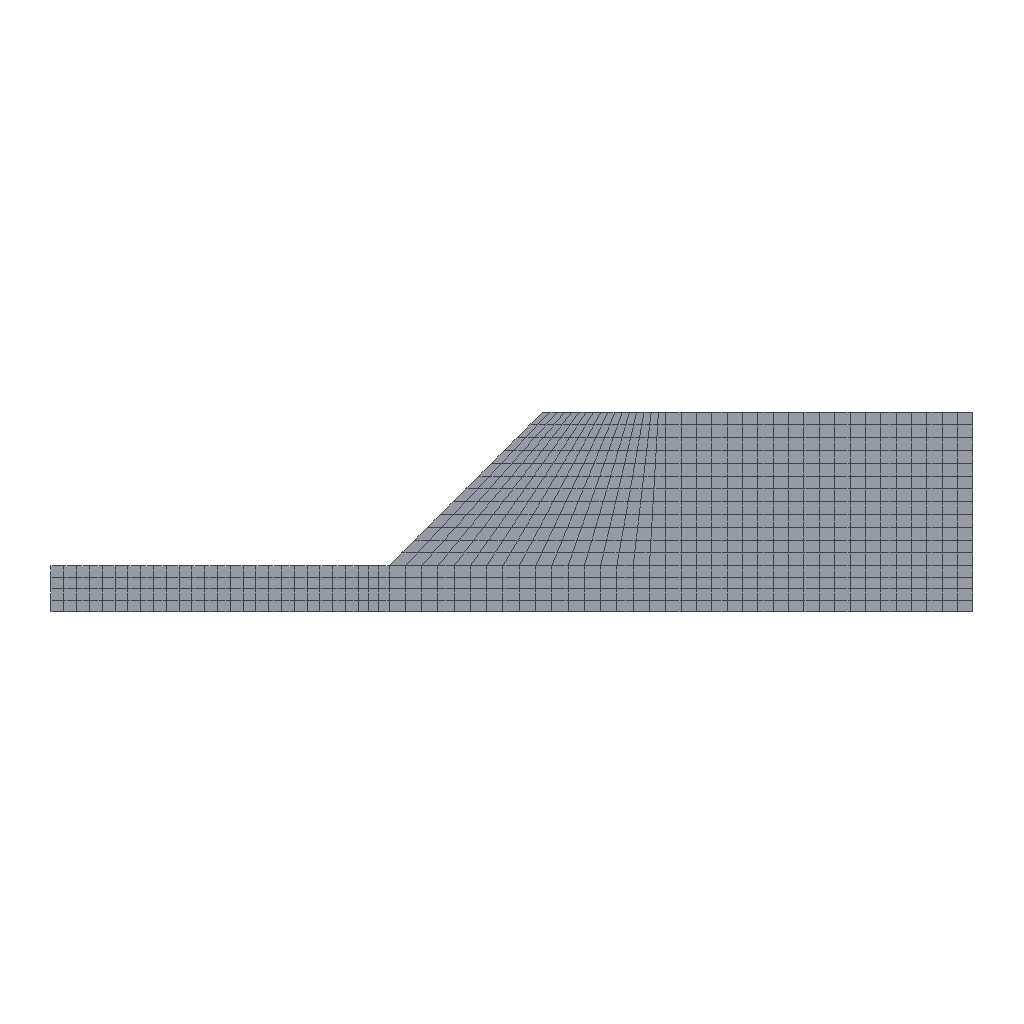Simulation study | abaqus
Set-up summary:
category,name,step,type,value,unit,region
solver,abaqus,,Abaqus/CAE 2024
units,mm-N-s-tonne (MPa),,inferred,E=10000 density=
analysis,Load,,static,time_period=1
analysis,Reduce,,static,time_period=1
mesh,nodes,,,781
mesh,elements,,,700
element_type,CPE4,,,700
material,soft,,E,10000
material,soft,,nu,0.35
material,soft,,behaviors,plastic; mohr coulomb; mohr coulomb hardening
material,soil,,E,100000
material,soil,,nu,0.35
material,soil,,behaviors,plastic; mohr coulomb; mohr coulomb hardening
section,soil,,solid section,,,_PickedSet17
section,soft,,solid section,,,_PickedSet18
load,,initial,initial condition field
load,Load-1,Load,by,-20,,_PickedSet7
bc,BC-1,initial,fixed,[dofs=x],,_PickedSet8
bc,BC-2,initial,fixed,"[dofs=x,y n=2]",,_PickedSet9
Abaqus input file, long lists of numbers shortened:
*Conflicts, Generated keywords
*Heading
** Job name: deck Model name: Model-1
** Generated by: Abaqus/CAE 2024
*Preprint, echo=NO, model=NO, history=NO, contact=NO
*Conflicts, User edited keywords
*Conflicts, End of conflict block
*Part, name=slope
*Node
      1,         -10.,           0.
      2,         -10.,           3.
** (779 more lines like these left out)
*Element, type=CPE4
 1,   1,  16, 217,  43
 2,  16,  17, 218, 217
** (698 more lines like these left out)
*Nset, nset=_PickedSet17, internal
   1,   2,   3,   4,   5,   6,   7,   8,   9,  11,  12,  15,  16,  17,  18,  19
  20,  21,  22,  23,  24,  25,  26,  27,  28,  29,  30,  31,  32,  33,  34,  35
** (39 more lines like these left out)
*Elset, elset=_PickedSet17, internal
   1,   2,   3,   4,   5,   6,   7,   8,   9,  10,  11,  12,  13,  14,  15,  16
  17,  18,  19,  20,  21,  22,  23,  24,  25,  26,  27,  28,  29,  30,  31,  32
** (34 more lines like these left out)
*Nset, nset=_PickedSet18, internal
   1,   2,   5,   6,   9,  10,  13,  14,  16,  17,  18,  44,  45,  46,  88,  89
  90,  91,  92,  93,  94,  95,  96,  97,  98,  99, 100, 101, 102, 103, 104, 105
** (9 more lines like these left out)
*Elset, elset=_PickedSet18, internal
 129, 130, 131, 132, 133, 134, 135, 136, 137, 138, 139, 140, 141, 142, 143, 144
 145, 146, 147, 148, 149, 150, 151, 152, 153, 154, 155, 156, 157, 158, 159, 160
** (6 more lines like these left out)
*Nset, nset=slope, generate
   1,  781,    1
*Elset, elset=slope, generate
   1,  700,    1
** Section: soil
*Solid Section, elset=_PickedSet17, material=soil
1.,
** Section: soft
*Solid Section, elset=_PickedSet18, material=soft
1.,
*End Part
**
**
** ASSEMBLY
**
*Assembly, name=Assembly
**
*Instance, name=slope-1, part=slope
*End Instance
**
*Nset, nset=_PickedSet7, internal, instance=slope-1, generate
   1,  781,    1
*Elset, elset=_PickedSet7, internal, instance=slope-1, generate
   1,  700,    1
*Nset, nset=_PickedSet8, internal, instance=slope-1
   3,   4,   7,   8,  12,  30,  31,  32,  66,  67,  68, 134, 135, 136, 137, 138
 139, 140, 141, 142, 143, 144
*Elset, elset=_PickedSet8, internal, instance=slope-1
  45,  46,  47,  48, 125, 126, 127, 128, 425, 426, 427, 428, 429, 430, 431, 432
 433, 434, 435, 436
*Nset, nset=_PickedSet9, internal, instance=slope-1
   1,   4,   6,   7,  10,  13,  33,  34,  35,  36,  37,  38,  39,  40,  41,  42
  43,  47,  48,  49,  50,  51,  52,  53,  54,  55,  56,  57,  58,  59,  60,  61
** (3 more lines like these left out)
*Elset, elset=_PickedSet9, internal, instance=slope-1
   1,   5,   9,  13,  17,  21,  25,  29,  33,  37,  41,  45,  52,  56,  60,  64
  68,  72,  76,  80,  84,  88,  92,  96, 100, 104, 108, 112, 116, 120, 124, 128
** (2 more lines like these left out)
*End Assembly
**
** MATERIALS
**
*Material, name=soft
*Elastic
10000., 0.35
*Mohr Coulomb, dependencies=1
0.,  0., , 0.5
0.,  0., ,  2.
*Mohr Coulomb Hardening, dependencies=1
40.,   0., , 0.25
10.,   0., ,   1.
 5.,   0., ,   2.
*Material, name=soil
*Elastic
100000., 0.35
*Mohr Coulomb, dependencies=1
   55.51,   0., , 0.25
 36.052,   0., ,  0.5
  25.887,   0., , 0.75
     20.,   0., ,   1.
 16.234,   0., , 1.25
  13.639,   0., ,  1.5
  11.749,   0., , 1.75
 10.314,   0., ,   2.
*Mohr Coulomb Hardening, dependencies=1
   49.52,   0., , 0.25
   24.76,   0., ,  0.5
 16.507,   0., , 0.75
   12.38,   0., ,   1.
   9.904,   0., , 1.25
 8.253,   0., ,  1.5
 7.074,   0., , 1.75
    6.19,   0., ,   2.
**
** BOUNDARY CONDITIONS
**
** Name: BC-1 Type: Displacement/Rotation
*Boundary
_PickedSet8, 1, 1
** Name: BC-2 Type: Displacement/Rotation
*Boundary
_PickedSet9, 1, 1
_PickedSet9, 2, 2
** ----------------------------------------------------------------
*initial conditions,type=field,VARIABLE=1
slope-1.slope,0.25
**
** STEP: Load
**
*Step, name=Load, nlgeom=NO, unsymm=YES
*Static
0.1, 1., 1e-05, 1.
**
** LOADS
**
** Name: Load-1   Type: Body force
*Dload
_PickedSet7, BY, -20.
**
** OUTPUT REQUESTS
**
*Restart, write, frequency=0
*Print, solve=NO
**
** FIELD OUTPUT: F-Output-1
**
*Output, field
*Node Output
CF, RF, U
*Element Output, directions=YES
FV, LE, PE, PEEQ, PEMAG, S
*Contact Output
CDISP, CSTRESS
**
** HISTORY OUTPUT: H-Output-1
**
*Output, history, variable=PRESELECT
*End Step
** ----------------------------------------------------------------
**
** STEP: Reduce
**
*Step, name=Reduce, nlgeom=NO, unsymm=YES
*Static
0.1, 1., 1e-05, 1.
*field,VARIABLE=1
slope-1.slope,1
**
** OUTPUT REQUESTS
**
*Restart, write, frequency=0
**
** FIELD OUTPUT: F-Output-1
**
*Output, field
*Node Output
CF, RF, U
*Element Output, directions=YES
FV, LE, PE, PEEQ, PEMAG, S
*Contact Output
CDISP, CSTRESS
**
** HISTORY OUTPUT: H-Output-1
**
*Output, history, variable=PRESELECT
*End Step
Results summary:
result,odb.job_status,,,JOB_STATUS_EXITED_WITH_ERROR,"consistent, unstated (Abaqus has no unit system)"
result,steps[0].procedure,Load,,*STATIC,"consistent, unstated (Abaqus has no unit system)"
result,steps[0].time_period,Load,,1,"consistent, unstated (Abaqus has no unit system)"
result,steps[0].n_frames,Load,,7,"consistent, unstated (Abaqus has no unit system)"
result,steps[0].last_frame.id,Load,,6,"consistent, unstated (Abaqus has no unit system)"
result,steps[0].last_frame.value,Load,,1,"consistent, unstated (Abaqus has no unit system)"
result,steps[0].last_frame.description,Load,,Increment      6: Step Time =    1.000,"consistent, unstated (Abaqus has no unit system)"
result,steps[0].completed,Load,,True,"consistent, unstated (Abaqus has no unit system)"
result,steps[0].max_U_magnitude,Load,,0.04148,"consistent, unstated (Abaqus has no unit system)"
result,steps[0].max_S_mises,Load,,407.582,"consistent, unstated (Abaqus has no unit system)"
result,steps[0].RF_sum[1],Load,,2.28882e-05,"consistent, unstated (Abaqus has no unit system)"
result,steps[0].RF_sum[2],Load,,10200,"consistent, unstated (Abaqus has no unit system)"
result,steps[1].procedure,Reduce,,*STATIC,"consistent, unstated (Abaqus has no unit system)"
result,steps[1].time_period,Reduce,,0.4724,"consistent, unstated (Abaqus has no unit system)"
result,steps[1].n_frames,Reduce,,39,"consistent, unstated (Abaqus has no unit system)"
result,steps[1].last_frame.id,Reduce,,38,"consistent, unstated (Abaqus has no unit system)"
result,steps[1].last_frame.value,Reduce,,0.4724,"consistent, unstated (Abaqus has no unit system)"
result,steps[1].last_frame.description,Reduce,,Increment     38: Step Time =   0.4724,"consistent, unstated (Abaqus has no unit system)"
result,steps[1].completed,Reduce,,True,"consistent, unstated (Abaqus has no unit system)"
result,steps[1].max_U_magnitude,Reduce,,0.1104,"consistent, unstated (Abaqus has no unit system)"
result,steps[1].max_S_mises,Reduce,,267.729,"consistent, unstated (Abaqus has no unit system)"
result,steps[1].RF_sum[1],Reduce,,-3.8147e-05,"consistent, unstated (Abaqus has no unit system)"
result,steps[1].RF_sum[2],Reduce,,10200,"consistent, unstated (Abaqus has no unit system)"